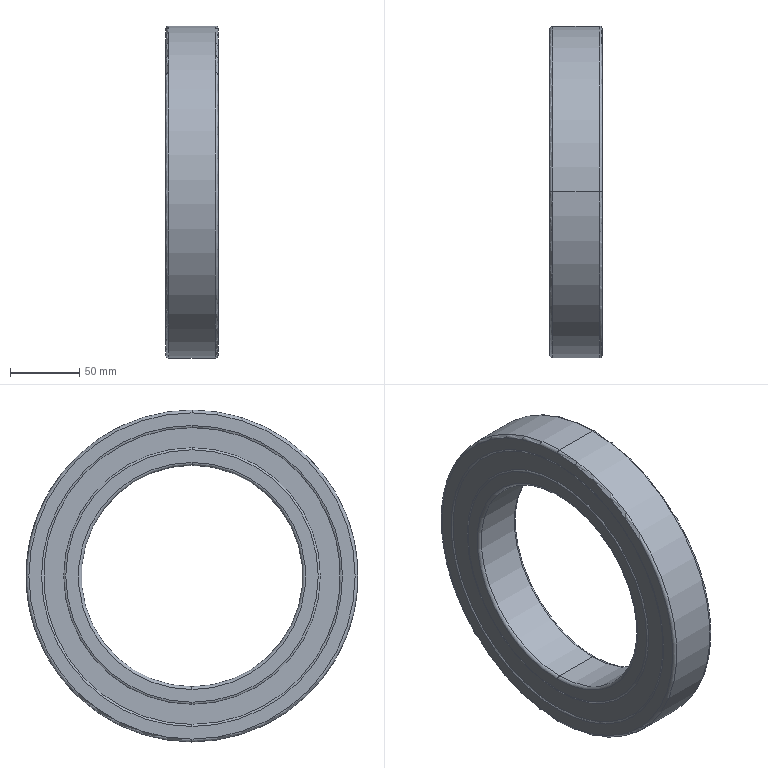Part | SolidWorks | features BaseBody 27 | 27 solids | 296 faces | box 38 x 240 x 240 mm | volume 735391 mm3 | cylinder 110 | sphere 102 | plane 58 | torus 26 | commonest cylinder face diameters 196 x49 204 x49 186.667 x4 213.333 x4 160 x2 240 x2